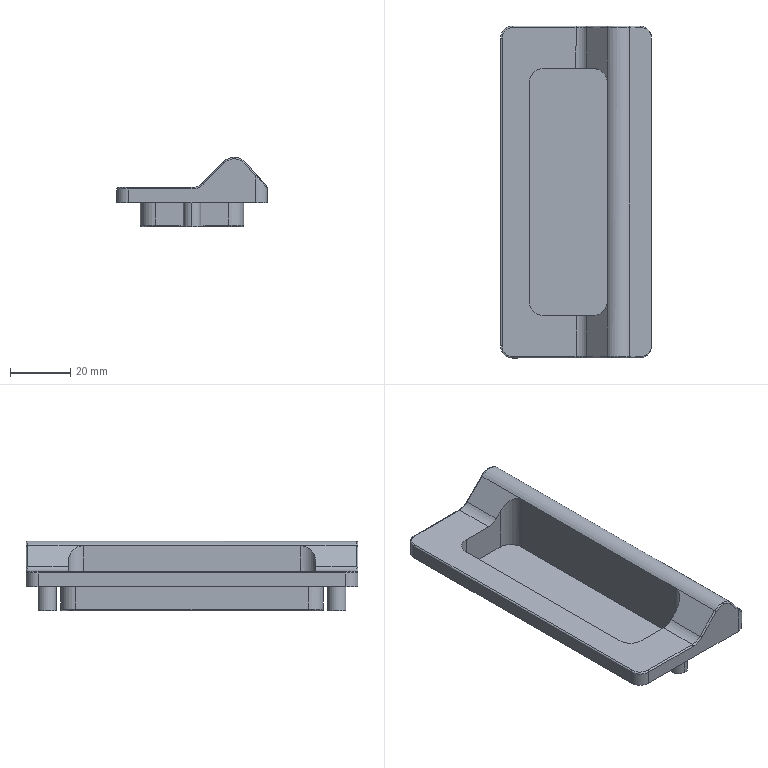Part | SolidWorks | features BaseBody 1 | 1 solid | 81 faces | box 50 x 110 x 23 mm | volume 40280 mm3 | cylinder 37 | plane 23 | spline 21 | commonest cylinder face diameters 1 x14 10 x11 3.2 x4 6 x4 8 x4